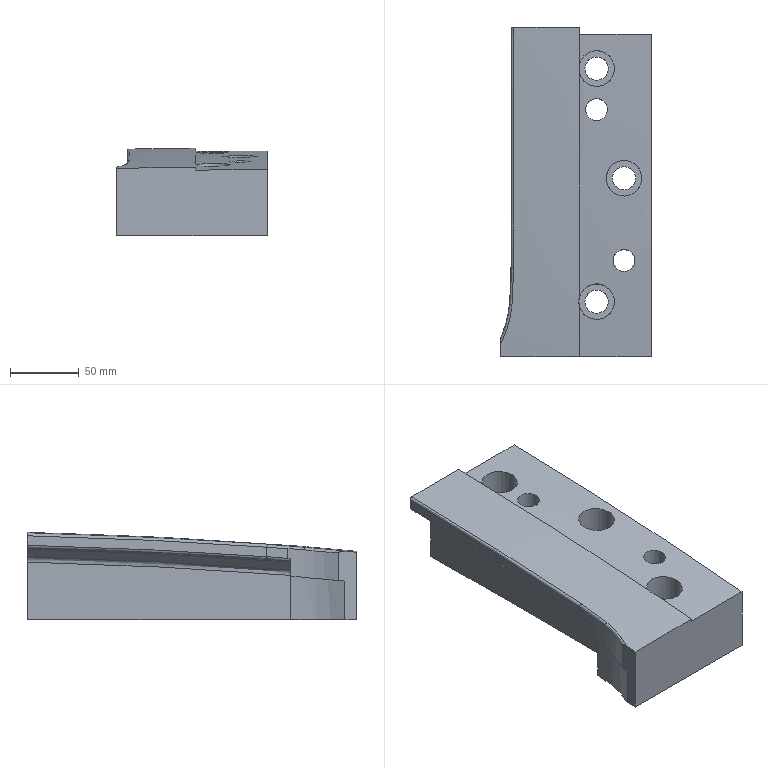Part | NX | features MAIN_BODY 2 | 1 solid | 41 faces | box 110 x 240 x 63.58 mm | volume 1105305 mm3 | spline 17 | plane 15 | cylinder 9 | commonest cylinder face diameters 17 x3 26 x3 16 x2 3.403 x1